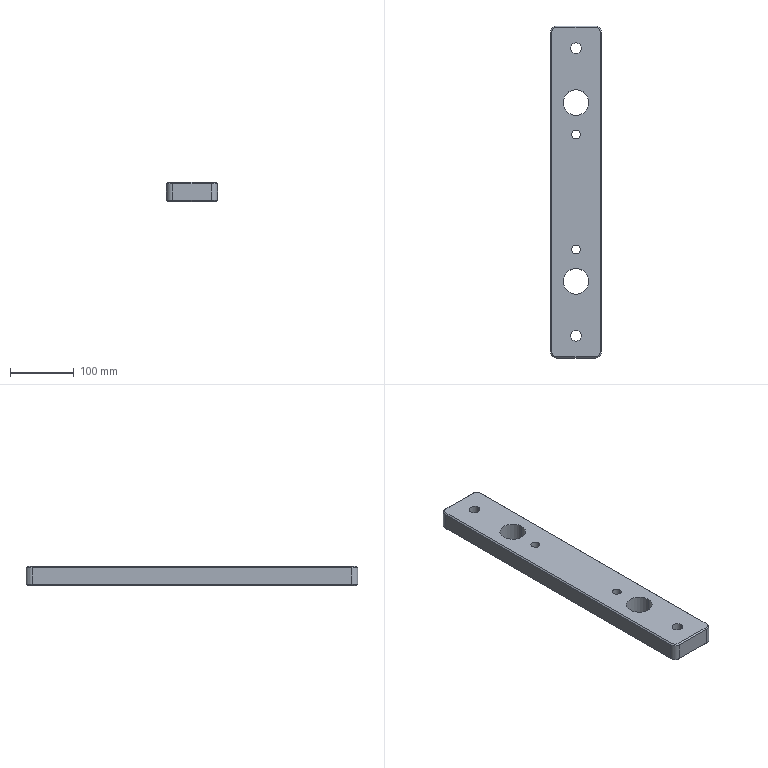Part | STEP file | TJ-DHQM-003-006 | 1 solid | 38 faces | box 80 x 520 x 30 mm | volume 1140560 mm3 | cylinder 16 | plane 14 | cone 8 | commonest cylinder face diameters 14 x4 17 x4 20 x4 40.5 x4
STEP:
#1=CARTESIAN_POINT('',(-7.,90.,0.));
#2=VERTEX_POINT('',#1);
#3=CARTESIAN_POINT('',(7.,90.,0.));
#4=VERTEX_POINT('',#3);
#5=CARTESIAN_POINT('',(0.,90.,0.));
#6=DIRECTION('',(0.,0.,1.));
#7=DIRECTION('',(1.,0.,0.));
#8=AXIS2_PLACEMENT_3D('',#5,#6,#7);
#9=CIRCLE('',#8,7.);
#10=EDGE_CURVE('',#2,#4,#9,.T.);
#11=ORIENTED_EDGE('',*,*,#10,.F.);
#12=CARTESIAN_POINT('',(-7.,90.,30.));
#13=VERTEX_POINT('',#12);
#14=CARTESIAN_POINT('',(-7.,90.,30.));
#15=DIRECTION('',(0.,0.,1.));
#16=VECTOR('',#15,1000.);
#17=LINE('',#14,#16);
#18=EDGE_CURVE('',#2,#13,#17,.T.);
#19=ORIENTED_EDGE('',*,*,#18,.T.);
#20=CARTESIAN_POINT('',(7.,90.,30.));
#21=VERTEX_POINT('',#20);
#22=CARTESIAN_POINT('',(0.,90.,30.));
#23=DIRECTION('',(0.,0.,1.));
#24=DIRECTION('',(1.,0.,0.));
#25=AXIS2_PLACEMENT_3D('',#22,#23,#24);
#26=CIRCLE('',#25,7.);
#27=EDGE_CURVE('',#13,#21,#26,.T.);
#28=ORIENTED_EDGE('',*,*,#27,.T.);
#29=CARTESIAN_POINT('',(7.,90.,30.));
#30=DIRECTION('',(0.,0.,1.));
#31=VECTOR('',#30,1000.);
#32=LINE('',#29,#31);
#33=EDGE_CURVE('',#4,#21,#32,.T.);
#34=ORIENTED_EDGE('',*,*,#33,.F.);
#35=EDGE_LOOP('',(#11,#19,#28,#34));
#36=FACE_OUTER_BOUND('',#35,.T.);
#37=CARTESIAN_POINT('',(0.,90.,30.));
#38=DIRECTION('',(0.,0.,1.));
#39=DIRECTION('',(1.,0.,0.));
#40=AXIS2_PLACEMENT_3D('',#37,#38,#39);
#41=CYLINDRICAL_SURFACE('',#40,7.);
#42=ADVANCED_FACE('',(#36),#41,.F.);
#43=CARTESIAN_POINT('',(-7.,-90.,0.));
#44=VERTEX_POINT('',#43);
#45=CARTESIAN_POINT('',(7.,-90.,0.));
#46=VERTEX_POINT('',#45);
#47=CARTESIAN_POINT('',(0.,-90.,0.));
#48=DIRECTION('',(0.,0.,1.));
#49=DIRECTION('',(1.,0.,0.));
#50=AXIS2_PLACEMENT_3D('',#47,#48,#49);
#51=CIRCLE('',#50,7.);
#52=EDGE_CURVE('',#44,#46,#51,.T.);
#53=ORIENTED_EDGE('',*,*,#52,.F.);
#54=CARTESIAN_POINT('',(-7.,-90.,30.));
#55=VERTEX_POINT('',#54);
#56=CARTESIAN_POINT('',(-7.,-90.,30.));
#57=DIRECTION('',(0.,0.,1.));
#58=VECTOR('',#57,1000.);
#59=LINE('',#56,#58);
#60=EDGE_CURVE('',#44,#55,#59,.T.);
#61=ORIENTED_EDGE('',*,*,#60,.T.);
#62=CARTESIAN_POINT('',(7.,-90.,30.));
#63=VERTEX_POINT('',#62);
#64=CARTESIAN_POINT('',(0.,-90.,30.));
#65=DIRECTION('',(0.,0.,1.));
#66=DIRECTION('',(1.,0.,0.));
#67=AXIS2_PLACEMENT_3D('',#64,#65,#66);
#68=CIRCLE('',#67,7.);
#69=EDGE_CURVE('',#55,#63,#68,.T.);
#70=ORIENTED_EDGE('',*,*,#69,.T.);
#71=CARTESIAN_POINT('',(7.,-90.,30.));
#72=DIRECTION('',(0.,0.,1.));
#73=VECTOR('',#72,1000.);
#74=LINE('',#71,#73);
#75=EDGE_CURVE('',#46,#63,#74,.T.);
#76=ORIENTED_EDGE('',*,*,#75,.F.);
#77=EDGE_LOOP('',(#53,#61,#70,#76));
#78=FACE_OUTER_BOUND('',#77,.T.);
#79=CARTESIAN_POINT('',(0.,-90.,30.));
#80=DIRECTION('',(0.,0.,1.));
#81=DIRECTION('',(1.,0.,0.));
#82=AXIS2_PLACEMENT_3D('',#79,#80,#81);
#83=CYLINDRICAL_SURFACE('',#82,7.);
#84=ADVANCED_FACE('',(#78),#83,.F.);
#85=CARTESIAN_POINT('',(20.25,140.,30.));
#86=VERTEX_POINT('',#85);
#87=CARTESIAN_POINT('',(-20.25,140.,30.));
#88=VERTEX_POINT('',#87);
#89=CARTESIAN_POINT('',(0.,140.,30.));
#90=DIRECTION('',(0.,0.,-1.));
#91=DIRECTION('',(-1.,0.,0.));
#92=AXIS2_PLACEMENT_3D('',#89,#90,#91);
#93=CIRCLE('',#92,20.25);
#94=EDGE_CURVE('',#86,#88,#93,.T.);
#95=ORIENTED_EDGE('',*,*,#94,.F.);
#96=CARTESIAN_POINT('',(20.25,140.,0.));
#97=VERTEX_POINT('',#96);
#98=CARTESIAN_POINT('',(20.25,140.,0.));
#99=DIRECTION('',(0.,0.,-1.));
#100=VECTOR('',#99,1000.);
#101=LINE('',#98,#100);
#102=EDGE_CURVE('',#86,#97,#101,.T.);
#103=ORIENTED_EDGE('',*,*,#102,.T.);
#104=CARTESIAN_POINT('',(-20.25,140.,0.));
#105=VERTEX_POINT('',#104);
#106=CARTESIAN_POINT('',(0.,140.,0.));
#107=DIRECTION('',(0.,0.,-1.));
#108=DIRECTION('',(-1.,0.,0.));
#109=AXIS2_PLACEMENT_3D('',#106,#107,#108);
#110=CIRCLE('',#109,20.25);
#111=EDGE_CURVE('',#97,#105,#110,.T.);
#112=ORIENTED_EDGE('',*,*,#111,.T.);
#113=CARTESIAN_POINT('',(-20.25,140.,0.));
#114=DIRECTION('',(0.,0.,-1.));
#115=VECTOR('',#114,1000.);
#116=LINE('',#113,#115);
#117=EDGE_CURVE('',#88,#105,#116,.T.);
#118=ORIENTED_EDGE('',*,*,#117,.F.);
#119=EDGE_LOOP('',(#95,#103,#112,#118));
#120=FACE_OUTER_BOUND('',#119,.T.);
#121=CARTESIAN_POINT('',(0.,140.,0.));
#122=DIRECTION('',(0.,0.,-1.));
#123=DIRECTION('',(-1.,0.,0.));
#124=AXIS2_PLACEMENT_3D('',#121,#122,#123);
#125=CYLINDRICAL_SURFACE('',#124,20.25);
#126=ADVANCED_FACE('',(#120),#125,.F.);
#127=CARTESIAN_POINT('',(20.25,-140.,30.));
#128=VERTEX_POINT('',#127);
#129=CARTESIAN_POINT('',(-20.25,-140.,30.));
#130=VERTEX_POINT('',#129);
#131=CARTESIAN_POINT('',(0.,-140.,30.));
#132=DIRECTION('',(0.,0.,-1.));
#133=DIRECTION('',(-1.,0.,0.));
#134=AXIS2_PLACEMENT_3D('',#131,#132,#133);
#135=CIRCLE('',#134,20.25);
#136=EDGE_CURVE('',#128,#130,#135,.T.);
#137=ORIENTED_EDGE('',*,*,#136,.F.);
#138=CARTESIAN_POINT('',(20.25,-140.,0.));
#139=VERTEX_POINT('',#138);
#140=CARTESIAN_POINT('',(20.25,-140.,0.));
#141=DIRECTION('',(0.,0.,-1.));
#142=VECTOR('',#141,1000.);
#143=LINE('',#140,#142);
#144=EDGE_CURVE('',#128,#139,#143,.T.);
#145=ORIENTED_EDGE('',*,*,#144,.T.);
#146=CARTESIAN_POINT('',(-20.25,-140.,0.));
#147=VERTEX_POINT('',#146);
#148=CARTESIAN_POINT('',(0.,-140.,0.));
#149=DIRECTION('',(0.,0.,-1.));
#150=DIRECTION('',(-1.,0.,0.));
#151=AXIS2_PLACEMENT_3D('',#148,#149,#150);
#152=CIRCLE('',#151,20.25);
#153=EDGE_CURVE('',#139,#147,#152,.T.);
#154=ORIENTED_EDGE('',*,*,#153,.T.);
#155=CARTESIAN_POINT('',(-20.25,-140.,0.));
#156=DIRECTION('',(0.,0.,-1.));
#157=VECTOR('',#156,1000.);
#158=LINE('',#155,#157);
#159=EDGE_CURVE('',#130,#147,#158,.T.);
#160=ORIENTED_EDGE('',*,*,#159,.F.);
#161=EDGE_LOOP('',(#137,#145,#154,#160));
#162=FACE_OUTER_BOUND('',#161,.T.);
#163=CARTESIAN_POINT('',(0.,-140.,0.));
#164=DIRECTION('',(0.,0.,-1.));
#165=DIRECTION('',(-1.,0.,0.));
#166=AXIS2_PLACEMENT_3D('',#163,#164,#165);
#167=CYLINDRICAL_SURFACE('',#166,20.25);
#168=ADVANCED_FACE('',(#162),#167,.F.);
#169=CARTESIAN_POINT('',(8.5,225.,30.));
#170=VERTEX_POINT('',#169);
#171=CARTESIAN_POINT('',(-8.5,225.,30.));
#172=VERTEX_POINT('',#171);
#173=CARTESIAN_POINT('',(0.,225.,30.));
#174=DIRECTION('',(0.,0.,-1.));
#175=DIRECTION('',(-1.,0.,0.));
#176=AXIS2_PLACEMENT_3D('',#173,#174,#175);
#177=CIRCLE('',#176,8.5);
#178=EDGE_CURVE('',#170,#172,#177,.T.);
#179=ORIENTED_EDGE('',*,*,#178,.F.);
#180=CARTESIAN_POINT('',(8.5,225.,0.));
#181=VERTEX_POINT('',#180);
#182=CARTESIAN_POINT('',(8.5,225.,30.));
#183=DIRECTION('',(0.,0.,-1.));
#184=VECTOR('',#183,1000.);
#185=LINE('',#182,#184);
#186=EDGE_CURVE('',#170,#181,#185,.T.);
#187=ORIENTED_EDGE('',*,*,#186,.T.);
#188=CARTESIAN_POINT('',(-8.5,225.,0.));
#189=VERTEX_POINT('',#188);
#190=CARTESIAN_POINT('',(0.,225.,0.));
#191=DIRECTION('',(0.,0.,-1.));
#192=DIRECTION('',(-1.,0.,0.));
#193=AXIS2_PLACEMENT_3D('',#190,#191,#192);
#194=CIRCLE('',#193,8.5);
#195=EDGE_CURVE('',#181,#189,#194,.T.);
#196=ORIENTED_EDGE('',*,*,#195,.T.);
#197=CARTESIAN_POINT('',(-8.5,225.,30.));
#198=DIRECTION('',(0.,0.,-1.));
#199=VECTOR('',#198,1000.);
#200=LINE('',#197,#199);
#201=EDGE_CURVE('',#172,#189,#200,.T.);
#202=ORIENTED_EDGE('',*,*,#201,.F.);
#203=EDGE_LOOP('',(#179,#187,#196,#202));
#204=FACE_OUTER_BOUND('',#203,.T.);
#205=CARTESIAN_POINT('',(0.,225.,30.));
#206=DIRECTION('',(0.,0.,-1.));
#207=DIRECTION('',(-1.,0.,0.));
#208=AXIS2_PLACEMENT_3D('',#205,#206,#207);
#209=CYLINDRICAL_SURFACE('',#208,8.5);
#210=ADVANCED_FACE('',(#204),#209,.F.);
#211=CARTESIAN_POINT('',(8.5,-225.,30.));
#212=VERTEX_POINT('',#211);
#213=CARTESIAN_POINT('',(-8.5,-225.,30.));
#214=VERTEX_POINT('',#213);
#215=CARTESIAN_POINT('',(0.,-225.,30.));
#216=DIRECTION('',(0.,0.,-1.));
#217=DIRECTION('',(-1.,0.,0.));
#218=AXIS2_PLACEMENT_3D('',#215,#216,#217);
#219=CIRCLE('',#218,8.5);
#220=EDGE_CURVE('',#212,#214,#219,.T.);
#221=ORIENTED_EDGE('',*,*,#220,.F.);
#222=CARTESIAN_POINT('',(8.5,-225.,0.));
#223=VERTEX_POINT('',#222);
#224=CARTESIAN_POINT('',(8.5,-225.,30.));
#225=DIRECTION('',(0.,0.,-1.));
#226=VECTOR('',#225,1000.);
#227=LINE('',#224,#226);
#228=EDGE_CURVE('',#212,#223,#227,.T.);
#229=ORIENTED_EDGE('',*,*,#228,.T.);
#230=CARTESIAN_POINT('',(-8.5,-225.,0.));
#231=VERTEX_POINT('',#230);
#232=CARTESIAN_POINT('',(0.,-225.,0.));
#233=DIRECTION('',(0.,0.,-1.));
#234=DIRECTION('',(-1.,0.,0.));
#235=AXIS2_PLACEMENT_3D('',#232,#233,#234);
#236=CIRCLE('',#235,8.5);
#237=EDGE_CURVE('',#223,#231,#236,.T.);
#238=ORIENTED_EDGE('',*,*,#237,.T.);
#239=CARTESIAN_POINT('',(-8.5,-225.,30.));
#240=DIRECTION('',(0.,0.,-1.));
#241=VECTOR('',#240,1000.);
#242=LINE('',#239,#241);
#243=EDGE_CURVE('',#214,#231,#242,.T.);
#244=ORIENTED_EDGE('',*,*,#243,.F.);
#245=EDGE_LOOP('',(#221,#229,#238,#244));
#246=FACE_OUTER_BOUND('',#245,.T.);
#247=CARTESIAN_POINT('',(0.,-225.,30.));
#248=DIRECTION('',(0.,0.,-1.));
#249=DIRECTION('',(-1.,0.,0.));
#250=AXIS2_PLACEMENT_3D('',#247,#248,#249);
#251=CYLINDRICAL_SURFACE('',#250,8.5);
#252=ADVANCED_FACE('',(#246),#251,.F.);
#253=CARTESIAN_POINT('',(40.,-250.,28.));
#254=VERTEX_POINT('',#253);
#255=CARTESIAN_POINT('',(40.,-250.,2.));
#256=VERTEX_POINT('',#255);
#257=CARTESIAN_POINT('',(40.,-250.,30.));
#258=DIRECTION('',(0.,0.,-1.));
#259=VECTOR('',#258,1000.);
#260=LINE('',#257,#259);
#261=EDGE_CURVE('',#254,#256,#260,.T.);
#262=ORIENTED_EDGE('',*,*,#261,.T.);
#263=CARTESIAN_POINT('',(40.,250.,2.));
#264=VERTEX_POINT('',#263);
#265=CARTESIAN_POINT('',(40.,260.,2.));
#266=DIRECTION('',(0.,1.,0.));
#267=VECTOR('',#266,1000.);
#268=LINE('',#265,#267);
#269=EDGE_CURVE('',#256,#264,#268,.T.);
#270=ORIENTED_EDGE('',*,*,#269,.T.);
#271=CARTESIAN_POINT('',(40.,250.,28.));
#272=VERTEX_POINT('',#271);
#273=CARTESIAN_POINT('',(40.,250.,30.));
#274=DIRECTION('',(0.,0.,1.));
#275=VECTOR('',#274,1000.);
#276=LINE('',#273,#275);
#277=EDGE_CURVE('',#264,#272,#276,.T.);
#278=ORIENTED_EDGE('',*,*,#277,.T.);
#279=CARTESIAN_POINT('',(40.,-250.,28.));
#280=DIRECTION('',(0.,-1.,0.));
#281=VECTOR('',#280,1000.);
#282=LINE('',#279,#281);
#283=EDGE_CURVE('',#272,#254,#282,.T.);
#284=ORIENTED_EDGE('',*,*,#283,.T.);
#285=EDGE_LOOP('',(#262,#270,#278,#284));
#286=FACE_OUTER_BOUND('',#285,.T.);
#287=CARTESIAN_POINT('',(40.,260.,30.));
#288=DIRECTION('',(-1.,0.,0.));
#289=DIRECTION('',(0.,-1.,0.));
#290=AXIS2_PLACEMENT_3D('',#287,#288,#289);
#291=PLANE('',#290);
#292=ADVANCED_FACE('',(#286),#291,.F.);
#293=CARTESIAN_POINT('',(30.,260.,28.));
#294=VERTEX_POINT('',#293);
#295=CARTESIAN_POINT('',(30.,260.,2.));
#296=VERTEX_POINT('',#295);
#297=CARTESIAN_POINT('',(30.,260.,30.));
#298=DIRECTION('',(0.,0.,-1.));
#299=VECTOR('',#298,1000.);
#300=LINE('',#297,#299);
#301=EDGE_CURVE('',#294,#296,#300,.T.);
#302=ORIENTED_EDGE('',*,*,#301,.T.);
#303=CARTESIAN_POINT('',(-30.,260.,2.));
#304=VERTEX_POINT('',#303);
#305=CARTESIAN_POINT('',(-40.,260.,2.));
#306=DIRECTION('',(-1.,0.,0.));
#307=VECTOR('',#306,1000.);
#308=LINE('',#305,#307);
#309=EDGE_CURVE('',#296,#304,#308,.T.);
#310=ORIENTED_EDGE('',*,*,#309,.T.);
#311=CARTESIAN_POINT('',(-30.,260.,28.));
#312=VERTEX_POINT('',#311);
#313=CARTESIAN_POINT('',(-30.,260.,30.));
#314=DIRECTION('',(0.,0.,1.));
#315=VECTOR('',#314,1000.);
#316=LINE('',#313,#315);
#317=EDGE_CURVE('',#304,#312,#316,.T.);
#318=ORIENTED_EDGE('',*,*,#317,.T.);
#319=CARTESIAN_POINT('',(30.,260.,28.));
#320=DIRECTION('',(1.,0.,0.));
#321=VECTOR('',#320,1000.);
#322=LINE('',#319,#321);
#323=EDGE_CURVE('',#312,#294,#322,.T.);
#324=ORIENTED_EDGE('',*,*,#323,.T.);
#325=EDGE_LOOP('',(#302,#310,#318,#324));
#326=FACE_OUTER_BOUND('',#325,.T.);
#327=CARTESIAN_POINT('',(-40.,260.,30.));
#328=DIRECTION('',(0.,-1.,0.));
#329=DIRECTION('',(0.,0.,-1.));
#330=AXIS2_PLACEMENT_3D('',#327,#328,#329);
#331=PLANE('',#330);
#332=ADVANCED_FACE('',(#326),#331,.F.);
#333=CARTESIAN_POINT('',(-40.,250.,28.));
#334=VERTEX_POINT('',#333);
#335=CARTESIAN_POINT('',(-40.,250.,2.));
#336=VERTEX_POINT('',#335);
#337=CARTESIAN_POINT('',(-40.,250.,30.));
#338=DIRECTION('',(0.,0.,-1.));
#339=VECTOR('',#338,1000.);
#340=LINE('',#337,#339);
#341=EDGE_CURVE('',#334,#336,#340,.T.);
#342=ORIENTED_EDGE('',*,*,#341,.T.);
#343=CARTESIAN_POINT('',(-40.,-250.,2.));
#344=VERTEX_POINT('',#343);
#345=CARTESIAN_POINT('',(-40.,260.,2.));
#346=DIRECTION('',(0.,-1.,0.));
#347=VECTOR('',#346,1000.);
#348=LINE('',#345,#347);
#349=EDGE_CURVE('',#336,#344,#348,.T.);
#350=ORIENTED_EDGE('',*,*,#349,.T.);
#351=CARTESIAN_POINT('',(-40.,-250.,28.));
#352=VERTEX_POINT('',#351);
#353=CARTESIAN_POINT('',(-40.,-250.,30.));
#354=DIRECTION('',(0.,0.,1.));
#355=VECTOR('',#354,1000.);
#356=LINE('',#353,#355);
#357=EDGE_CURVE('',#344,#352,#356,.T.);
#358=ORIENTED_EDGE('',*,*,#357,.T.);
#359=CARTESIAN_POINT('',(-40.,250.,28.));
#360=DIRECTION('',(0.,1.,0.));
#361=VECTOR('',#360,1000.);
#362=LINE('',#359,#361);
#363=EDGE_CURVE('',#352,#334,#362,.T.);
#364=ORIENTED_EDGE('',*,*,#363,.T.);
#365=EDGE_LOOP('',(#342,#350,#358,#364));
#366=FACE_OUTER_BOUND('',#365,.T.);
#367=CARTESIAN_POINT('',(-40.,260.,30.));
#368=DIRECTION('',(1.,0.,0.));
#369=DIRECTION('',(0.,1.,0.));
#370=AXIS2_PLACEMENT_3D('',#367,#368,#369);
#371=PLANE('',#370);
#372=ADVANCED_FACE('',(#366),#371,.F.);
#373=CARTESIAN_POINT('',(-30.,-260.,28.));
#374=VERTEX_POINT('',#373);
#375=CARTESIAN_POINT('',(-30.,-260.,2.));
#376=VERTEX_POINT('',#375);
#377=CARTESIAN_POINT('',(-30.,-260.,30.));
#378=DIRECTION('',(0.,0.,-1.));
#379=VECTOR('',#378,1000.);
#380=LINE('',#377,#379);
#381=EDGE_CURVE('',#374,#376,#380,.T.);
#382=ORIENTED_EDGE('',*,*,#381,.T.);
#383=CARTESIAN_POINT('',(30.,-260.,2.));
#384=VERTEX_POINT('',#383);
#385=CARTESIAN_POINT('',(-40.,-260.,2.));
#386=DIRECTION('',(1.,0.,0.));
#387=VECTOR('',#386,1000.);
#388=LINE('',#385,#387);
#389=EDGE_CURVE('',#376,#384,#388,.T.);
#390=ORIENTED_EDGE('',*,*,#389,.T.);
#391=CARTESIAN_POINT('',(30.,-260.,28.));
#392=VERTEX_POINT('',#391);
#393=CARTESIAN_POINT('',(30.,-260.,30.));
#394=DIRECTION('',(0.,0.,1.));
#395=VECTOR('',#394,1000.);
#396=LINE('',#393,#395);
#397=EDGE_CURVE('',#384,#392,#396,.T.);
#398=ORIENTED_EDGE('',*,*,#397,.T.);
#399=CARTESIAN_POINT('',(-30.,-260.,28.));
#400=DIRECTION('',(-1.,0.,0.));
#401=VECTOR('',#400,1000.);
#402=LINE('',#399,#401);
#403=EDGE_CURVE('',#392,#374,#402,.T.);
#404=ORIENTED_EDGE('',*,*,#403,.T.);
#405=EDGE_LOOP('',(#382,#390,#398,#404));
#406=FACE_OUTER_BOUND('',#405,.T.);
#407=CARTESIAN_POINT('',(-40.,-260.,30.));
#408=DIRECTION('',(0.,1.,0.));
#409=DIRECTION('',(0.,0.,1.));
#410=AXIS2_PLACEMENT_3D('',#407,#408,#409);
#411=PLANE('',#410);
#412=ADVANCED_FACE('',(#406),#411,.F.);
#413=CARTESIAN_POINT('',(38.,-250.,30.));
#414=VERTEX_POINT('',#413);
#415=CARTESIAN_POINT('',(38.,250.,30.));
#416=VERTEX_POINT('',#415);
#417=CARTESIAN_POINT('',(38.,250.,30.));
#418=DIRECTION('',(0.,1.,0.));
#419=VECTOR('',#418,1000.);
#420=LINE('',#417,#419);
#421=EDGE_CURVE('',#414,#416,#420,.T.);
#422=ORIENTED_EDGE('',*,*,#421,.T.);
#423=CARTESIAN_POINT('',(30.,258.,30.));
#424=VERTEX_POINT('',#423);
#425=CARTESIAN_POINT('',(30.,250.,30.));
#426=DIRECTION('',(0.,0.,1.));
#427=DIRECTION('',(1.,0.,0.));
#428=AXIS2_PLACEMENT_3D('',#425,#426,#427);
#429=CIRCLE('',#428,8.);
#430=EDGE_CURVE('',#416,#424,#429,.T.);
#431=ORIENTED_EDGE('',*,*,#430,.T.);
#432=CARTESIAN_POINT('',(-30.,258.,30.));
#433=VERTEX_POINT('',#432);
#434=CARTESIAN_POINT('',(-30.,258.,30.));
#435=DIRECTION('',(-1.,0.,0.));
#436=VECTOR('',#435,1000.);
#437=LINE('',#434,#436);
#438=EDGE_CURVE('',#424,#433,#437,.T.);
#439=ORIENTED_EDGE('',*,*,#438,.T.);
#440=CARTESIAN_POINT('',(-38.,250.,30.));
#441=VERTEX_POINT('',#440);
#442=CARTESIAN_POINT('',(-30.,250.,30.));
#443=DIRECTION('',(0.,0.,1.));
#444=DIRECTION('',(1.,0.,0.));
#445=AXIS2_PLACEMENT_3D('',#442,#443,#444);
#446=CIRCLE('',#445,8.);
#447=EDGE_CURVE('',#433,#441,#446,.T.);
#448=ORIENTED_EDGE('',*,*,#447,.T.);
#449=CARTESIAN_POINT('',(-38.,-250.,30.));
#450=VERTEX_POINT('',#449);
#451=CARTESIAN_POINT('',(-38.,-250.,30.));
#452=DIRECTION('',(0.,-1.,0.));
#453=VECTOR('',#452,1000.);
#454=LINE('',#451,#453);
#455=EDGE_CURVE('',#441,#450,#454,.T.);
#456=ORIENTED_EDGE('',*,*,#455,.T.);
#457=CARTESIAN_POINT('',(-30.,-258.,30.));
#458=VERTEX_POINT('',#457);
#459=CARTESIAN_POINT('',(-30.,-250.,30.));
#460=DIRECTION('',(0.,0.,1.));
#461=DIRECTION('',(1.,0.,0.));
#462=AXIS2_PLACEMENT_3D('',#459,#460,#461);
#463=CIRCLE('',#462,8.);
#464=EDGE_CURVE('',#450,#458,#463,.T.);
#465=ORIENTED_EDGE('',*,*,#464,.T.);
#466=CARTESIAN_POINT('',(30.,-258.,30.));
#467=VERTEX_POINT('',#466);
#468=CARTESIAN_POINT('',(30.,-258.,30.));
#469=DIRECTION('',(1.,0.,0.));
#470=VECTOR('',#469,1000.);
#471=LINE('',#468,#470);
#472=EDGE_CURVE('',#458,#467,#471,.T.);
#473=ORIENTED_EDGE('',*,*,#472,.T.);
#474=CARTESIAN_POINT('',(30.,-250.,30.));
#475=DIRECTION('',(0.,0.,1.));
#476=DIRECTION('',(1.,0.,0.));
#477=AXIS2_PLACEMENT_3D('',#474,#475,#476);
#478=CIRCLE('',#477,8.);
#479=EDGE_CURVE('',#467,#414,#478,.T.);
#480=ORIENTED_EDGE('',*,*,#479,.T.);
#481=EDGE_LOOP('',(#422,#431,#439,#448,#456,#465,#473,#480));
#482=FACE_OUTER_BOUND('',#481,.T.);
#483=CARTESIAN_POINT('',(0.,90.,30.));
#484=DIRECTION('',(0.,0.,1.));
#485=DIRECTION('',(1.,0.,0.));
#486=AXIS2_PLACEMENT_3D('',#483,#484,#485);
#487=CIRCLE('',#486,7.);
#488=EDGE_CURVE('',#21,#13,#487,.T.);
#489=ORIENTED_EDGE('',*,*,#488,.F.);
#490=ORIENTED_EDGE('',*,*,#27,.F.);
#491=EDGE_LOOP('',(#489,#490));
#492=FACE_BOUND('',#491,.T.);
#493=CARTESIAN_POINT('',(0.,-90.,30.));
#494=DIRECTION('',(0.,0.,1.));
#495=DIRECTION('',(1.,0.,0.));
#496=AXIS2_PLACEMENT_3D('',#493,#494,#495);
#497=CIRCLE('',#496,7.);
#498=EDGE_CURVE('',#63,#55,#497,.T.);
#499=ORIENTED_EDGE('',*,*,#498,.F.);
#500=ORIENTED_EDGE('',*,*,#69,.F.);
#501=EDGE_LOOP('',(#499,#500));
#502=FACE_BOUND('',#501,.T.);
#503=CARTESIAN_POINT('',(0.,140.,30.));
#504=DIRECTION('',(0.,0.,-1.));
#505=DIRECTION('',(-1.,0.,0.));
#506=AXIS2_PLACEMENT_3D('',#503,#504,#505);
#507=CIRCLE('',#506,20.25);
#508=EDGE_CURVE('',#88,#86,#507,.T.);
#509=ORIENTED_EDGE('',*,*,#508,.T.);
#510=ORIENTED_EDGE('',*,*,#94,.T.);
#511=EDGE_LOOP('',(#509,#510));
#512=FACE_BOUND('',#511,.T.);
#513=CARTESIAN_POINT('',(0.,-140.,30.));
#514=DIRECTION('',(0.,0.,-1.));
#515=DIRECTION('',(-1.,0.,0.));
#516=AXIS2_PLACEMENT_3D('',#513,#514,#515);
#517=CIRCLE('',#516,20.25);
#518=EDGE_CURVE('',#130,#128,#517,.T.);
#519=ORIENTED_EDGE('',*,*,#518,.T.);
#520=ORIENTED_EDGE('',*,*,#136,.T.);
#521=EDGE_LOOP('',(#519,#520));
#522=FACE_BOUND('',#521,.T.);
#523=CARTESIAN_POINT('',(0.,225.,30.));
#524=DIRECTION('',(0.,0.,-1.));
#525=DIRECTION('',(-1.,0.,0.));
#526=AXIS2_PLACEMENT_3D('',#523,#524,#525);
#527=CIRCLE('',#526,8.5);
#528=EDGE_CURVE('',#172,#170,#527,.T.);
#529=ORIENTED_EDGE('',*,*,#528,.T.);
#530=ORIENTED_EDGE('',*,*,#178,.T.);
#531=EDGE_LOOP('',(#529,#530));
#532=FACE_BOUND('',#531,.T.);
#533=CARTESIAN_POINT('',(0.,-225.,30.));
#534=DIRECTION('',(0.,0.,-1.));
#535=DIRECTION('',(-1.,0.,0.));
#536=AXIS2_PLACEMENT_3D('',#533,#534,#535);
#537=CIRCLE('',#536,8.5);
#538=EDGE_CURVE('',#214,#212,#537,.T.);
#539=ORIENTED_EDGE('',*,*,#538,.T.);
#540=ORIENTED_EDGE('',*,*,#220,.T.);
#541=EDGE_LOOP('',(#539,#540));
#542=FACE_BOUND('',#541,.T.);
#543=CARTESIAN_POINT('',(0.,0.,30.));
#544=DIRECTION('',(0.,0.,1.));
#545=DIRECTION('',(1.,0.,0.));
#546=AXIS2_PLACEMENT_3D('',#543,#544,#545);
#547=PLANE('',#546);
#548=ADVANCED_FACE('',(#482,#492,#502,#512,#522,#532,#542),#547,.T.);
#549=CARTESIAN_POINT('',(-30.,258.,0.));
#550=VERTEX_POINT('',#549);
#551=CARTESIAN_POINT('',(30.,258.,0.));
#552=VERTEX_POINT('',#551);
#553=CARTESIAN_POINT('',(0.,258.,0.));
#554=DIRECTION('',(1.,0.,0.));
#555=VECTOR('',#554,1000.);
#556=LINE('',#553,#555);
#557=EDGE_CURVE('',#550,#552,#556,.T.);
#558=ORIENTED_EDGE('',*,*,#557,.T.);
#559=CARTESIAN_POINT('',(38.,250.,0.));
#560=VERTEX_POINT('',#559);
#561=CARTESIAN_POINT('',(30.,250.,0.));
#562=DIRECTION('',(0.,0.,-1.));
#563=DIRECTION('',(1.,0.,0.));
#564=AXIS2_PLACEMENT_3D('',#561,#562,#563);
#565=CIRCLE('',#564,8.);
#566=EDGE_CURVE('',#552,#560,#565,.T.);
#567=ORIENTED_EDGE('',*,*,#566,.T.);
#568=CARTESIAN_POINT('',(38.,-250.,0.));
#569=VERTEX_POINT('',#568);
#570=CARTESIAN_POINT('',(38.,0.,0.));
#571=DIRECTION('',(0.,-1.,0.));
#572=VECTOR('',#571,1000.);
#573=LINE('',#570,#572);
#574=EDGE_CURVE('',#560,#569,#573,.T.);
#575=ORIENTED_EDGE('',*,*,#574,.T.);
#576=CARTESIAN_POINT('',(30.,-258.,0.));
#577=VERTEX_POINT('',#576);
#578=CARTESIAN_POINT('',(30.,-250.,0.));
#579=DIRECTION('',(0.,0.,-1.));
#580=DIRECTION('',(1.,0.,0.));
#581=AXIS2_PLACEMENT_3D('',#578,#579,#580);
#582=CIRCLE('',#581,8.);
#583=EDGE_CURVE('',#569,#577,#582,.T.);
#584=ORIENTED_EDGE('',*,*,#583,.T.);
#585=CARTESIAN_POINT('',(-30.,-258.,0.));
#586=VERTEX_POINT('',#585);
#587=CARTESIAN_POINT('',(0.,-258.,0.));
#588=DIRECTION('',(-1.,0.,0.));
#589=VECTOR('',#588,1000.);
#590=LINE('',#587,#589);
#591=EDGE_CURVE('',#577,#586,#590,.T.);
#592=ORIENTED_EDGE('',*,*,#591,.T.);
#593=CARTESIAN_POINT('',(-38.,-250.,0.));
#594=VERTEX_POINT('',#593);
#595=CARTESIAN_POINT('',(-30.,-250.,0.));
#596=DIRECTION('',(0.,0.,-1.));
#597=DIRECTION('',(1.,0.,0.));
#598=AXIS2_PLACEMENT_3D('',#595,#596,#597);
#599=CIRCLE('',#598,8.);
#600=EDGE_CURVE('',#586,#594,#599,.T.);
#601=ORIENTED_EDGE('',*,*,#600,.T.);
#602=CARTESIAN_POINT('',(-38.,250.,0.));
#603=VERTEX_POINT('',#602);
#604=CARTESIAN_POINT('',(-38.,0.,0.));
#605=DIRECTION('',(0.,1.,0.));
#606=VECTOR('',#605,1000.);
#607=LINE('',#604,#606);
#608=EDGE_CURVE('',#594,#603,#607,.T.);
#609=ORIENTED_EDGE('',*,*,#608,.T.);
#610=CARTESIAN_POINT('',(-30.,250.,0.));
#611=DIRECTION('',(0.,0.,-1.));
#612=DIRECTION('',(1.,0.,0.));
#613=AXIS2_PLACEMENT_3D('',#610,#611,#612);
#614=CIRCLE('',#613,8.);
#615=EDGE_CURVE('',#603,#550,#614,.T.);
#616=ORIENTED_EDGE('',*,*,#615,.T.);
#617=EDGE_LOOP('',(#558,#567,#575,#584,#592,#601,#609,#616));
#618=FACE_OUTER_BOUND('',#617,.T.);
#619=CARTESIAN_POINT('',(0.,90.,0.));
#620=DIRECTION('',(0.,0.,1.));
#621=DIRECTION('',(1.,0.,0.));
#622=AXIS2_PLACEMENT_3D('',#619,#620,#621);
#623=CIRCLE('',#622,7.);
#624=EDGE_CURVE('',#4,#2,#623,.T.);
#625=ORIENTED_EDGE('',*,*,#624,.T.);
#626=ORIENTED_EDGE('',*,*,#10,.T.);
#627=EDGE_LOOP('',(#625,#626));
#628=FACE_BOUND('',#627,.T.);
#629=CARTESIAN_POINT('',(0.,-90.,0.));
#630=DIRECTION('',(0.,0.,1.));
#631=DIRECTION('',(1.,0.,0.));
#632=AXIS2_PLACEMENT_3D('',#629,#630,#631);
#633=CIRCLE('',#632,7.);
#634=EDGE_CURVE('',#46,#44,#633,.T.);
#635=ORIENTED_EDGE('',*,*,#634,.T.);
#636=ORIENTED_EDGE('',*,*,#52,.T.);
#637=EDGE_LOOP('',(#635,#636));
#638=FACE_BOUND('',#637,.T.);
#639=CARTESIAN_POINT('',(0.,140.,0.));
#640=DIRECTION('',(0.,0.,-1.));
#641=DIRECTION('',(-1.,0.,0.));
#642=AXIS2_PLACEMENT_3D('',#639,#640,#641);
#643=CIRCLE('',#642,20.25);
#644=EDGE_CURVE('',#105,#97,#643,.T.);
#645=ORIENTED_EDGE('',*,*,#644,.F.);
#646=ORIENTED_EDGE('',*,*,#111,.F.);
#647=EDGE_LOOP('',(#645,#646));
#648=FACE_BOUND('',#647,.T.);
#649=CARTESIAN_POINT('',(0.,-140.,0.));
#650=DIRECTION('',(0.,0.,-1.));
#651=DIRECTION('',(-1.,0.,0.));
#652=AXIS2_PLACEMENT_3D('',#649,#650,#651);
#653=CIRCLE('',#652,20.25);
#654=EDGE_CURVE('',#147,#139,#653,.T.);
#655=ORIENTED_EDGE('',*,*,#654,.F.);
#656=ORIENTED_EDGE('',*,*,#153,.F.);
#657=EDGE_LOOP('',(#655,#656));
#658=FACE_BOUND('',#657,.T.);
#659=CARTESIAN_POINT('',(0.,225.,0.));
#660=DIRECTION('',(0.,0.,-1.));
#661=DIRECTION('',(-1.,0.,0.));
#662=AXIS2_PLACEMENT_3D('',#659,#660,#661);
#663=CIRCLE('',#662,8.5);
#664=EDGE_CURVE('',#189,#181,#663,.T.);
#665=ORIENTED_EDGE('',*,*,#664,.F.);
#666=ORIENTED_EDGE('',*,*,#195,.F.);
#667=EDGE_LOOP('',(#665,#666));
#668=FACE_BOUND('',#667,.T.);
#669=CARTESIAN_POINT('',(0.,-225.,0.));
#670=DIRECTION('',(0.,0.,-1.));
#671=DIRECTION('',(-1.,0.,0.));
#672=AXIS2_PLACEMENT_3D('',#669,#670,#671);
#673=CIRCLE('',#672,8.5);
#674=EDGE_CURVE('',#231,#223,#673,.T.);
#675=ORIENTED_EDGE('',*,*,#674,.F.);
#676=ORIENTED_EDGE('',*,*,#237,.F.);
#677=EDGE_LOOP('',(#675,#676));
#678=FACE_BOUND('',#677,.T.);
#679=CARTESIAN_POINT('',(0.,0.,0.));
#680=DIRECTION('',(0.,0.,1.));
#681=DIRECTION('',(1.,0.,0.));
#682=AXIS2_PLACEMENT_3D('',#679,#680,#681);
#683=PLANE('',#682);
#684=ADVANCED_FACE('',(#618,#628,#638,#648,#658,#668,#678),#683,.F.);
#685=ORIENTED_EDGE('',*,*,#317,.F.);
#686=CARTESIAN_POINT('',(-30.,250.,2.));
#687=DIRECTION('',(0.,0.,1.));
#688=DIRECTION('',(1.,0.,0.));
#689=AXIS2_PLACEMENT_3D('',#686,#687,#688);
#690=CIRCLE('',#689,10.);
#691=EDGE_CURVE('',#304,#336,#690,.T.);
#692=ORIENTED_EDGE('',*,*,#691,.T.);
#693=ORIENTED_EDGE('',*,*,#341,.F.);
#694=CARTESIAN_POINT('',(-30.,250.,28.));
#695=DIRECTION('',(0.,0.,-1.));
#696=DIRECTION('',(1.,0.,0.));
#697=AXIS2_PLACEMENT_3D('',#694,#695,#696);
#698=CIRCLE('',#697,10.);
#699=EDGE_CURVE('',#334,#312,#698,.T.);
#700=ORIENTED_EDGE('',*,*,#699,.T.);
#701=EDGE_LOOP('',(#685,#692,#693,#700));
#702=FACE_OUTER_BOUND('',#701,.T.);
#703=CARTESIAN_POINT('',(-30.,250.,30.));
#704=DIRECTION('',(0.,0.,-1.));
#705=DIRECTION('',(-1.,0.,0.));
#706=AXIS2_PLACEMENT_3D('',#703,#704,#705);
#707=CYLINDRICAL_SURFACE('',#706,10.);
#708=ADVANCED_FACE('',(#702),#707,.T.);
#709=ORIENTED_EDGE('',*,*,#277,.F.);
#710=CARTESIAN_POINT('',(30.,250.,2.));
#711=DIRECTION('',(0.,0.,1.));
#712=DIRECTION('',(1.,0.,0.));
#713=AXIS2_PLACEMENT_3D('',#710,#711,#712);
#714=CIRCLE('',#713,10.);
#715=EDGE_CURVE('',#264,#296,#714,.T.);
#716=ORIENTED_EDGE('',*,*,#715,.T.);
#717=ORIENTED_EDGE('',*,*,#301,.F.);
#718=CARTESIAN_POINT('',(30.,250.,28.));
#719=DIRECTION('',(0.,0.,-1.));
#720=DIRECTION('',(1.,0.,0.));
#721=AXIS2_PLACEMENT_3D('',#718,#719,#720);
#722=CIRCLE('',#721,10.);
#723=EDGE_CURVE('',#294,#272,#722,.T.);
#724=ORIENTED_EDGE('',*,*,#723,.T.);
#725=EDGE_LOOP('',(#709,#716,#717,#724));
#726=FACE_OUTER_BOUND('',#725,.T.);
#727=CARTESIAN_POINT('',(30.,250.,30.));
#728=DIRECTION('',(0.,0.,-1.));
#729=DIRECTION('',(-1.,0.,0.));
#730=AXIS2_PLACEMENT_3D('',#727,#728,#729);
#731=CYLINDRICAL_SURFACE('',#730,10.);
#732=ADVANCED_FACE('',(#726),#731,.T.);
#733=ORIENTED_EDGE('',*,*,#357,.F.);
#734=CARTESIAN_POINT('',(-30.,-250.,2.));
#735=DIRECTION('',(0.,0.,1.));
#736=DIRECTION('',(1.,0.,0.));
#737=AXIS2_PLACEMENT_3D('',#734,#735,#736);
#738=CIRCLE('',#737,10.);
#739=EDGE_CURVE('',#344,#376,#738,.T.);
#740=ORIENTED_EDGE('',*,*,#739,.T.);
#741=ORIENTED_EDGE('',*,*,#381,.F.);
#742=CARTESIAN_POINT('',(-30.,-250.,28.));
#743=DIRECTION('',(0.,0.,-1.));
#744=DIRECTION('',(1.,0.,0.));
#745=AXIS2_PLACEMENT_3D('',#742,#743,#744);
#746=CIRCLE('',#745,10.);
#747=EDGE_CURVE('',#374,#352,#746,.T.);
#748=ORIENTED_EDGE('',*,*,#747,.T.);
#749=EDGE_LOOP('',(#733,#740,#741,#748));
#750=FACE_OUTER_BOUND('',#749,.T.);
#751=CARTESIAN_POINT('',(-30.,-250.,30.));
#752=DIRECTION('',(0.,0.,-1.));
#753=DIRECTION('',(-1.,0.,0.));
#754=AXIS2_PLACEMENT_3D('',#751,#752,#753);
#755=CYLINDRICAL_SURFACE('',#754,10.);
#756=ADVANCED_FACE('',(#750),#755,.T.);
#757=ORIENTED_EDGE('',*,*,#397,.F.);
#758=CARTESIAN_POINT('',(30.,-250.,2.));
#759=DIRECTION('',(0.,0.,1.));
#760=DIRECTION('',(1.,0.,0.));
#761=AXIS2_PLACEMENT_3D('',#758,#759,#760);
#762=CIRCLE('',#761,10.);
#763=EDGE_CURVE('',#384,#256,#762,.T.);
#764=ORIENTED_EDGE('',*,*,#763,.T.);
#765=ORIENTED_EDGE('',*,*,#261,.F.);
#766=CARTESIAN_POINT('',(30.,-250.,28.));
#767=DIRECTION('',(0.,0.,-1.));
#768=DIRECTION('',(1.,0.,0.));
#769=AXIS2_PLACEMENT_3D('',#766,#767,#768);
#770=CIRCLE('',#769,10.);
#771=EDGE_CURVE('',#254,#392,#770,.T.);
#772=ORIENTED_EDGE('',*,*,#771,.T.);
#773=EDGE_LOOP('',(#757,#764,#765,#772));
#774=FACE_OUTER_BOUND('',#773,.T.);
#775=CARTESIAN_POINT('',(30.,-250.,30.));
#776=DIRECTION('',(0.,0.,-1.));
#777=DIRECTION('',(-1.,0.,0.));
#778=AXIS2_PLACEMENT_3D('',#775,#776,#777);
#779=CYLINDRICAL_SURFACE('',#778,10.);
#780=ADVANCED_FACE('',(#774),#779,.T.);
#781=ORIENTED_EDGE('',*,*,#228,.F.);
#782=ORIENTED_EDGE('',*,*,#538,.F.);
#783=ORIENTED_EDGE('',*,*,#243,.T.);
#784=ORIENTED_EDGE('',*,*,#674,.T.);
#785=EDGE_LOOP('',(#781,#782,#783,#784));
#786=FACE_OUTER_BOUND('',#785,.T.);
#787=CARTESIAN_POINT('',(0.,-225.,30.));
#788=DIRECTION('',(0.,0.,-1.));
#789=DIRECTION('',(-1.,0.,0.));
#790=AXIS2_PLACEMENT_3D('',#787,#788,#789);
#791=CYLINDRICAL_SURFACE('',#790,8.5);
#792=ADVANCED_FACE('',(#786),#791,.F.);
#793=ORIENTED_EDGE('',*,*,#186,.F.);
#794=ORIENTED_EDGE('',*,*,#528,.F.);
#795=ORIENTED_EDGE('',*,*,#201,.T.);
#796=ORIENTED_EDGE('',*,*,#664,.T.);
#797=EDGE_LOOP('',(#793,#794,#795,#796));
#798=FACE_OUTER_BOUND('',#797,.T.);
#799=CARTESIAN_POINT('',(0.,225.,30.));
#800=DIRECTION('',(0.,0.,-1.));
#801=DIRECTION('',(-1.,0.,0.));
#802=AXIS2_PLACEMENT_3D('',#799,#800,#801);
#803=CYLINDRICAL_SURFACE('',#802,8.5);
#804=ADVANCED_FACE('',(#798),#803,.F.);
#805=ORIENTED_EDGE('',*,*,#144,.F.);
#806=ORIENTED_EDGE('',*,*,#518,.F.);
#807=ORIENTED_EDGE('',*,*,#159,.T.);
#808=ORIENTED_EDGE('',*,*,#654,.T.);
#809=EDGE_LOOP('',(#805,#806,#807,#808));
#810=FACE_OUTER_BOUND('',#809,.T.);
#811=CARTESIAN_POINT('',(0.,-140.,0.));
#812=DIRECTION('',(0.,0.,-1.));
#813=DIRECTION('',(-1.,0.,0.));
#814=AXIS2_PLACEMENT_3D('',#811,#812,#813);
#815=CYLINDRICAL_SURFACE('',#814,20.25);
#816=ADVANCED_FACE('',(#810),#815,.F.);
#817=ORIENTED_EDGE('',*,*,#102,.F.);
#818=ORIENTED_EDGE('',*,*,#508,.F.);
#819=ORIENTED_EDGE('',*,*,#117,.T.);
#820=ORIENTED_EDGE('',*,*,#644,.T.);
#821=EDGE_LOOP('',(#817,#818,#819,#820));
#822=FACE_OUTER_BOUND('',#821,.T.);
#823=CARTESIAN_POINT('',(0.,140.,0.));
#824=DIRECTION('',(0.,0.,-1.));
#825=DIRECTION('',(-1.,0.,0.));
#826=AXIS2_PLACEMENT_3D('',#823,#824,#825);
#827=CYLINDRICAL_SURFACE('',#826,20.25);
#828=ADVANCED_FACE('',(#822),#827,.F.);
#829=ORIENTED_EDGE('',*,*,#60,.F.);
#830=ORIENTED_EDGE('',*,*,#634,.F.);
#831=ORIENTED_EDGE('',*,*,#75,.T.);
#832=ORIENTED_EDGE('',*,*,#498,.T.);
#833=EDGE_LOOP('',(#829,#830,#831,#832));
#834=FACE_OUTER_BOUND('',#833,.T.);
#835=CARTESIAN_POINT('',(0.,-90.,30.));
#836=DIRECTION('',(0.,0.,1.));
#837=DIRECTION('',(1.,0.,0.));
#838=AXIS2_PLACEMENT_3D('',#835,#836,#837);
#839=CYLINDRICAL_SURFACE('',#838,7.);
#840=ADVANCED_FACE('',(#834),#839,.F.);
#841=ORIENTED_EDGE('',*,*,#18,.F.);
#842=ORIENTED_EDGE('',*,*,#624,.F.);
#843=ORIENTED_EDGE('',*,*,#33,.T.);
#844=ORIENTED_EDGE('',*,*,#488,.T.);
#845=EDGE_LOOP('',(#841,#842,#843,#844));
#846=FACE_OUTER_BOUND('',#845,.T.);
#847=CARTESIAN_POINT('',(0.,90.,30.));
#848=DIRECTION('',(0.,0.,1.));
#849=DIRECTION('',(1.,0.,0.));
#850=AXIS2_PLACEMENT_3D('',#847,#848,#849);
#851=CYLINDRICAL_SURFACE('',#850,7.);
#852=ADVANCED_FACE('',(#846),#851,.F.);
#853=CARTESIAN_POINT('',(-30.,-260.,2.));
#854=DIRECTION('',(0.,0.7071,-0.7071));
#855=VECTOR('',#854,1000.);
#856=LINE('',#853,#855);
#857=EDGE_CURVE('',#376,#586,#856,.T.);
#858=ORIENTED_EDGE('',*,*,#857,.F.);
#859=ORIENTED_EDGE('',*,*,#739,.F.);
#860=CARTESIAN_POINT('',(-38.,-250.,0.));
#861=DIRECTION('',(-0.7071,0.,0.7071));
#862=VECTOR('',#861,1000.);
#863=LINE('',#860,#862);
#864=EDGE_CURVE('',#594,#344,#863,.T.);
#865=ORIENTED_EDGE('',*,*,#864,.F.);
#866=ORIENTED_EDGE('',*,*,#600,.F.);
#867=EDGE_LOOP('',(#858,#859,#865,#866));
#868=FACE_OUTER_BOUND('',#867,.T.);
#869=CARTESIAN_POINT('',(-30.,-250.,0.));
#870=DIRECTION('',(0.,0.,1.));
#871=DIRECTION('',(1.,0.,0.));
#872=AXIS2_PLACEMENT_3D('',#869,#870,#871);
#873=CONICAL_SURFACE('',#872,8.,0.7854);
#874=ADVANCED_FACE('',(#868),#873,.T.);
#875=ORIENTED_EDGE('',*,*,#864,.T.);
#876=ORIENTED_EDGE('',*,*,#349,.F.);
#877=CARTESIAN_POINT('',(-38.,250.,0.));
#878=DIRECTION('',(-0.7071,0.,0.7071));
#879=VECTOR('',#878,1000.);
#880=LINE('',#877,#879);
#881=EDGE_CURVE('',#603,#336,#880,.T.);
#882=ORIENTED_EDGE('',*,*,#881,.F.);
#883=ORIENTED_EDGE('',*,*,#608,.F.);
#884=EDGE_LOOP('',(#875,#876,#882,#883));
#885=FACE_OUTER_BOUND('',#884,.T.);
#886=CARTESIAN_POINT('',(-40.,260.,2.));
#887=DIRECTION('',(0.7071,0.,0.7071));
#888=DIRECTION('',(0.,-1.,0.));
#889=AXIS2_PLACEMENT_3D('',#886,#887,#888);
#890=PLANE('',#889);
#891=ADVANCED_FACE('',(#885),#890,.F.);
#892=ORIENTED_EDGE('',*,*,#857,.T.);
#893=ORIENTED_EDGE('',*,*,#591,.F.);
#894=CARTESIAN_POINT('',(30.,-260.,2.));
#895=DIRECTION('',(0.,0.7071,-0.7071));
#896=VECTOR('',#895,1000.);
#897=LINE('',#894,#896);
#898=EDGE_CURVE('',#384,#577,#897,.T.);
#899=ORIENTED_EDGE('',*,*,#898,.F.);
#900=ORIENTED_EDGE('',*,*,#389,.F.);
#901=EDGE_LOOP('',(#892,#893,#899,#900));
#902=FACE_OUTER_BOUND('',#901,.T.);
#903=CARTESIAN_POINT('',(-40.,-260.,2.));
#904=DIRECTION('',(0.,0.7071,0.7071));
#905=DIRECTION('',(1.,0.,0.));
#906=AXIS2_PLACEMENT_3D('',#903,#904,#905);
#907=PLANE('',#906);
#908=ADVANCED_FACE('',(#902),#907,.F.);
#909=ORIENTED_EDGE('',*,*,#881,.T.);
#910=ORIENTED_EDGE('',*,*,#691,.F.);
#911=CARTESIAN_POINT('',(-30.,258.,0.));
#912=DIRECTION('',(0.,0.7071,0.7071));
#913=VECTOR('',#912,1000.);
#914=LINE('',#911,#913);
#915=EDGE_CURVE('',#550,#304,#914,.T.);
#916=ORIENTED_EDGE('',*,*,#915,.F.);
#917=ORIENTED_EDGE('',*,*,#615,.F.);
#918=EDGE_LOOP('',(#909,#910,#916,#917));
#919=FACE_OUTER_BOUND('',#918,.T.);
#920=CARTESIAN_POINT('',(-30.,250.,0.));
#921=DIRECTION('',(0.,0.,1.));
#922=DIRECTION('',(1.,0.,0.));
#923=AXIS2_PLACEMENT_3D('',#920,#921,#922);
#924=CONICAL_SURFACE('',#923,8.,0.7854);
#925=ADVANCED_FACE('',(#919),#924,.T.);
#926=ORIENTED_EDGE('',*,*,#898,.T.);
#927=ORIENTED_EDGE('',*,*,#583,.F.);
#928=CARTESIAN_POINT('',(40.,-250.,2.));
#929=DIRECTION('',(-0.7071,0.,-0.7071));
#930=VECTOR('',#929,1000.);
#931=LINE('',#928,#930);
#932=EDGE_CURVE('',#256,#569,#931,.T.);
#933=ORIENTED_EDGE('',*,*,#932,.F.);
#934=ORIENTED_EDGE('',*,*,#763,.F.);
#935=EDGE_LOOP('',(#926,#927,#933,#934));
#936=FACE_OUTER_BOUND('',#935,.T.);
#937=CARTESIAN_POINT('',(30.,-250.,0.));
#938=DIRECTION('',(0.,0.,1.));
#939=DIRECTION('',(1.,0.,0.));
#940=AXIS2_PLACEMENT_3D('',#937,#938,#939);
#941=CONICAL_SURFACE('',#940,8.,0.7854);
#942=ADVANCED_FACE('',(#936),#941,.T.);
#943=ORIENTED_EDGE('',*,*,#915,.T.);
#944=ORIENTED_EDGE('',*,*,#309,.F.);
#945=CARTESIAN_POINT('',(30.,258.,0.));
#946=DIRECTION('',(0.,0.7071,0.7071));
#947=VECTOR('',#946,1000.);
#948=LINE('',#945,#947);
#949=EDGE_CURVE('',#552,#296,#948,.T.);
#950=ORIENTED_EDGE('',*,*,#949,.F.);
#951=ORIENTED_EDGE('',*,*,#557,.F.);
#952=EDGE_LOOP('',(#943,#944,#950,#951));
#953=FACE_OUTER_BOUND('',#952,.T.);
#954=CARTESIAN_POINT('',(-40.,260.,2.));
#955=DIRECTION('',(0.,-0.7071,0.7071));
#956=DIRECTION('',(-1.,0.,0.));
#957=AXIS2_PLACEMENT_3D('',#954,#955,#956);
#958=PLANE('',#957);
#959=ADVANCED_FACE('',(#953),#958,.F.);
#960=ORIENTED_EDGE('',*,*,#932,.T.);
#961=ORIENTED_EDGE('',*,*,#574,.F.);
#962=CARTESIAN_POINT('',(40.,250.,2.));
#963=DIRECTION('',(-0.7071,0.,-0.7071));
#964=VECTOR('',#963,1000.);
#965=LINE('',#962,#964);
#966=EDGE_CURVE('',#264,#560,#965,.T.);
#967=ORIENTED_EDGE('',*,*,#966,.F.);
#968=ORIENTED_EDGE('',*,*,#269,.F.);
#969=EDGE_LOOP('',(#960,#961,#967,#968));
#970=FACE_OUTER_BOUND('',#969,.T.);
#971=CARTESIAN_POINT('',(40.,260.,2.));
#972=DIRECTION('',(-0.7071,0.,0.7071));
#973=DIRECTION('',(0.,1.,0.));
#974=AXIS2_PLACEMENT_3D('',#971,#972,#973);
#975=PLANE('',#974);
#976=ADVANCED_FACE('',(#970),#975,.F.);
#977=ORIENTED_EDGE('',*,*,#949,.T.);
#978=ORIENTED_EDGE('',*,*,#715,.F.);
#979=ORIENTED_EDGE('',*,*,#966,.T.);
#980=ORIENTED_EDGE('',*,*,#566,.F.);
#981=EDGE_LOOP('',(#977,#978,#979,#980));
#982=FACE_OUTER_BOUND('',#981,.T.);
#983=CARTESIAN_POINT('',(30.,250.,0.));
#984=DIRECTION('',(0.,0.,1.));
#985=DIRECTION('',(1.,0.,0.));
#986=AXIS2_PLACEMENT_3D('',#983,#984,#985);
#987=CONICAL_SURFACE('',#986,8.,0.7854);
#988=ADVANCED_FACE('',(#982),#987,.T.);
#989=CARTESIAN_POINT('',(-40.,-250.,28.));
#990=DIRECTION('',(0.7071,0.,0.7071));
#991=VECTOR('',#990,1000.);
#992=LINE('',#989,#991);
#993=EDGE_CURVE('',#352,#450,#992,.T.);
#994=ORIENTED_EDGE('',*,*,#993,.F.);
#995=ORIENTED_EDGE('',*,*,#747,.F.);
#996=CARTESIAN_POINT('',(-30.,-258.,30.));
#997=DIRECTION('',(0.,-0.7071,-0.7071));
#998=VECTOR('',#997,1000.);
#999=LINE('',#996,#998);
#1000=EDGE_CURVE('',#458,#374,#999,.T.);
#1001=ORIENTED_EDGE('',*,*,#1000,.F.);
#1002=ORIENTED_EDGE('',*,*,#464,.F.);
#1003=EDGE_LOOP('',(#994,#995,#1001,#1002));
#1004=FACE_OUTER_BOUND('',#1003,.T.);
#1005=CARTESIAN_POINT('',(-30.,-250.,30.));
#1006=DIRECTION('',(0.,0.,-1.));
#1007=DIRECTION('',(-1.,0.,0.));
#1008=AXIS2_PLACEMENT_3D('',#1005,#1006,#1007);
#1009=CONICAL_SURFACE('',#1008,8.,0.7854);
#1010=ADVANCED_FACE('',(#1004),#1009,.T.);
#1011=ORIENTED_EDGE('',*,*,#1000,.T.);
#1012=ORIENTED_EDGE('',*,*,#403,.F.);
#1013=CARTESIAN_POINT('',(30.,-258.,30.));
#1014=DIRECTION('',(0.,-0.7071,-0.7071));
#1015=VECTOR('',#1014,1000.);
#1016=LINE('',#1013,#1015);
#1017=EDGE_CURVE('',#467,#392,#1016,.T.);
#1018=ORIENTED_EDGE('',*,*,#1017,.F.);
#1019=ORIENTED_EDGE('',*,*,#472,.F.);
#1020=EDGE_LOOP('',(#1011,#1012,#1018,#1019));
#1021=FACE_OUTER_BOUND('',#1020,.T.);
#1022=CARTESIAN_POINT('',(0.,-258.,30.));
#1023=DIRECTION('',(0.,-0.7071,0.7071));
#1024=DIRECTION('',(-1.,0.,0.));
#1025=AXIS2_PLACEMENT_3D('',#1022,#1023,#1024);
#1026=PLANE('',#1025);
#1027=ADVANCED_FACE('',(#1021),#1026,.T.);
#1028=ORIENTED_EDGE('',*,*,#993,.T.);
#1029=ORIENTED_EDGE('',*,*,#455,.F.);
#1030=CARTESIAN_POINT('',(-40.,250.,28.));
#1031=DIRECTION('',(0.7071,0.,0.7071));
#1032=VECTOR('',#1031,1000.);
#1033=LINE('',#1030,#1032);
#1034=EDGE_CURVE('',#334,#441,#1033,.T.);
#1035=ORIENTED_EDGE('',*,*,#1034,.F.);
#1036=ORIENTED_EDGE('',*,*,#363,.F.);
#1037=EDGE_LOOP('',(#1028,#1029,#1035,#1036));
#1038=FACE_OUTER_BOUND('',#1037,.T.);
#1039=CARTESIAN_POINT('',(-38.,0.,30.));
#1040=DIRECTION('',(-0.7071,0.,0.7071));
#1041=DIRECTION('',(0.,1.,0.));
#1042=AXIS2_PLACEMENT_3D('',#1039,#1040,#1041);
#1043=PLANE('',#1042);
#1044=ADVANCED_FACE('',(#1038),#1043,.T.);
#1045=ORIENTED_EDGE('',*,*,#1017,.T.);
#1046=ORIENTED_EDGE('',*,*,#771,.F.);
#1047=CARTESIAN_POINT('',(38.,-250.,30.));
#1048=DIRECTION('',(0.7071,0.,-0.7071));
#1049=VECTOR('',#1048,1000.);
#1050=LINE('',#1047,#1049);
#1051=EDGE_CURVE('',#414,#254,#1050,.T.);
#1052=ORIENTED_EDGE('',*,*,#1051,.F.);
#1053=ORIENTED_EDGE('',*,*,#479,.F.);
#1054=EDGE_LOOP('',(#1045,#1046,#1052,#1053));
#1055=FACE_OUTER_BOUND('',#1054,.T.);
#1056=CARTESIAN_POINT('',(30.,-250.,30.));
#1057=DIRECTION('',(0.,0.,-1.));
#1058=DIRECTION('',(-1.,0.,0.));
#1059=AXIS2_PLACEMENT_3D('',#1056,#1057,#1058);
#1060=CONICAL_SURFACE('',#1059,8.,0.7854);
#1061=ADVANCED_FACE('',(#1055),#1060,.T.);
#1062=ORIENTED_EDGE('',*,*,#1034,.T.);
#1063=ORIENTED_EDGE('',*,*,#447,.F.);
#1064=CARTESIAN_POINT('',(-30.,260.,28.));
#1065=DIRECTION('',(0.,-0.7071,0.7071));
#1066=VECTOR('',#1065,1000.);
#1067=LINE('',#1064,#1066);
#1068=EDGE_CURVE('',#312,#433,#1067,.T.);
#1069=ORIENTED_EDGE('',*,*,#1068,.F.);
#1070=ORIENTED_EDGE('',*,*,#699,.F.);
#1071=EDGE_LOOP('',(#1062,#1063,#1069,#1070));
#1072=FACE_OUTER_BOUND('',#1071,.T.);
#1073=CARTESIAN_POINT('',(-30.,250.,30.));
#1074=DIRECTION('',(0.,0.,-1.));
#1075=DIRECTION('',(-1.,0.,0.));
#1076=AXIS2_PLACEMENT_3D('',#1073,#1074,#1075);
#1077=CONICAL_SURFACE('',#1076,8.,0.7854);
#1078=ADVANCED_FACE('',(#1072),#1077,.T.);
#1079=ORIENTED_EDGE('',*,*,#1051,.T.);
#1080=ORIENTED_EDGE('',*,*,#283,.F.);
#1081=CARTESIAN_POINT('',(38.,250.,30.));
#1082=DIRECTION('',(0.7071,0.,-0.7071));
#1083=VECTOR('',#1082,1000.);
#1084=LINE('',#1081,#1083);
#1085=EDGE_CURVE('',#416,#272,#1084,.T.);
#1086=ORIENTED_EDGE('',*,*,#1085,.F.);
#1087=ORIENTED_EDGE('',*,*,#421,.F.);
#1088=EDGE_LOOP('',(#1079,#1080,#1086,#1087));
#1089=FACE_OUTER_BOUND('',#1088,.T.);
#1090=CARTESIAN_POINT('',(38.,0.,30.));
#1091=DIRECTION('',(0.7071,0.,0.7071));
#1092=DIRECTION('',(0.,-1.,0.));
#1093=AXIS2_PLACEMENT_3D('',#1090,#1091,#1092);
#1094=PLANE('',#1093);
#1095=ADVANCED_FACE('',(#1089),#1094,.T.);
#1096=ORIENTED_EDGE('',*,*,#1068,.T.);
#1097=ORIENTED_EDGE('',*,*,#438,.F.);
#1098=CARTESIAN_POINT('',(30.,260.,28.));
#1099=DIRECTION('',(0.,-0.7071,0.7071));
#1100=VECTOR('',#1099,1000.);
#1101=LINE('',#1098,#1100);
#1102=EDGE_CURVE('',#294,#424,#1101,.T.);
#1103=ORIENTED_EDGE('',*,*,#1102,.F.);
#1104=ORIENTED_EDGE('',*,*,#323,.F.);
#1105=EDGE_LOOP('',(#1096,#1097,#1103,#1104));
#1106=FACE_OUTER_BOUND('',#1105,.T.);
#1107=CARTESIAN_POINT('',(0.,258.,30.));
#1108=DIRECTION('',(0.,0.7071,0.7071));
#1109=DIRECTION('',(1.,0.,0.));
#1110=AXIS2_PLACEMENT_3D('',#1107,#1108,#1109);
#1111=PLANE('',#1110);
#1112=ADVANCED_FACE('',(#1106),#1111,.T.);
#1113=ORIENTED_EDGE('',*,*,#1085,.T.);
#1114=ORIENTED_EDGE('',*,*,#723,.F.);
#1115=ORIENTED_EDGE('',*,*,#1102,.T.);
#1116=ORIENTED_EDGE('',*,*,#430,.F.);
#1117=EDGE_LOOP('',(#1113,#1114,#1115,#1116));
#1118=FACE_OUTER_BOUND('',#1117,.T.);
#1119=CARTESIAN_POINT('',(30.,250.,30.));
#1120=DIRECTION('',(0.,0.,-1.));
#1121=DIRECTION('',(-1.,0.,0.));
#1122=AXIS2_PLACEMENT_3D('',#1119,#1120,#1121);
#1123=CONICAL_SURFACE('',#1122,8.,0.7854);
#1124=ADVANCED_FACE('',(#1118),#1123,.T.);
#1125=CLOSED_SHELL('',(#42,#84,#126,#168,#210,#252,#292,#332,#372,#412,#548,#684,#708,#732,#756,#780,#792,#804,#816,#828,#840,#852,#874,#891,#908,#925,#942,#959,#976,#988,#1010,#1027,#1044,#1061,#1078,#1095,#1112,#1124));
#1126=MANIFOLD_SOLID_BREP('',#1125);
#1127=CARTESIAN_POINT('',(0.,0.,0.));
#1128=DIRECTION('',(0.,0.,1.));
#1129=DIRECTION('',(1.,0.,0.));
#1130=AXIS2_PLACEMENT_3D('',#1127,#1128,#1129);
#1131=(LENGTH_UNIT()NAMED_UNIT(*)SI_UNIT(.MILLI.,.METRE.));
#1132=UNCERTAINTY_MEASURE_WITH_UNIT(LENGTH_MEASURE(0.00001),#1131,'','');
#1133=(NAMED_UNIT(*)PLANE_ANGLE_UNIT()SI_UNIT($,.RADIAN.));
#1134=(NAMED_UNIT(*)SI_UNIT($,.STERADIAN.)SOLID_ANGLE_UNIT());
#1135=(GEOMETRIC_REPRESENTATION_CONTEXT(3)GLOBAL_UNCERTAINTY_ASSIGNED_CONTEXT((#1132))GLOBAL_UNIT_ASSIGNED_CONTEXT((#1131,#1133,#1134))REPRESENTATION_CONTEXT('',''));
#1136=ADVANCED_BREP_SHAPE_REPRESENTATION('',(#1126,#1130),#1135);